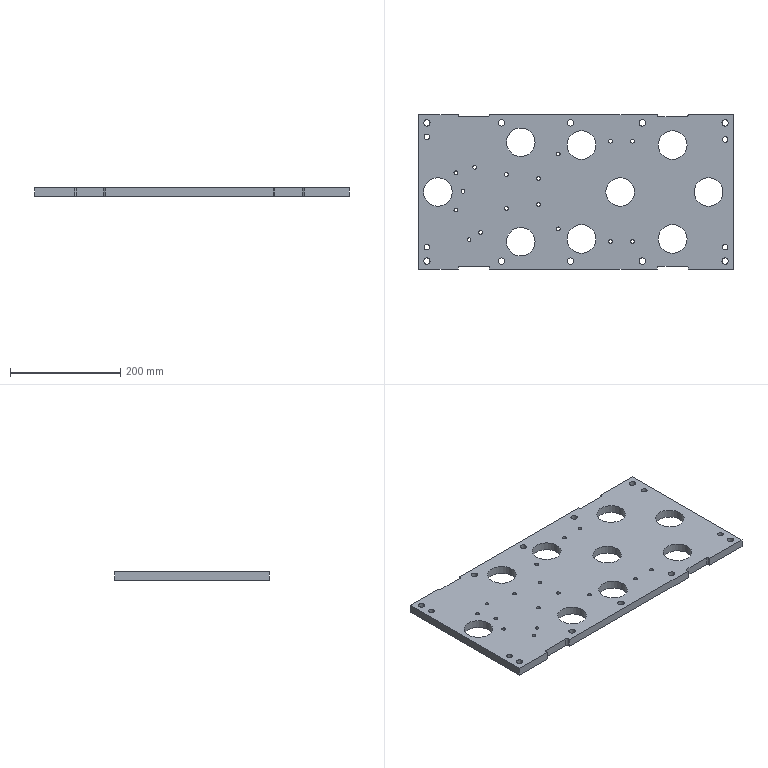Part | NX | features UB-2 2 | 1 solid | 86 faces | box 570 x 280 x 15 mm | volume 2061578 mm3 | cylinder 48 | plane 22 | cone 16 | commonest cylinder face diameters 6.806 x15 11.507 x10 52.004 x9 6 x8 10 x4 6.8 x1